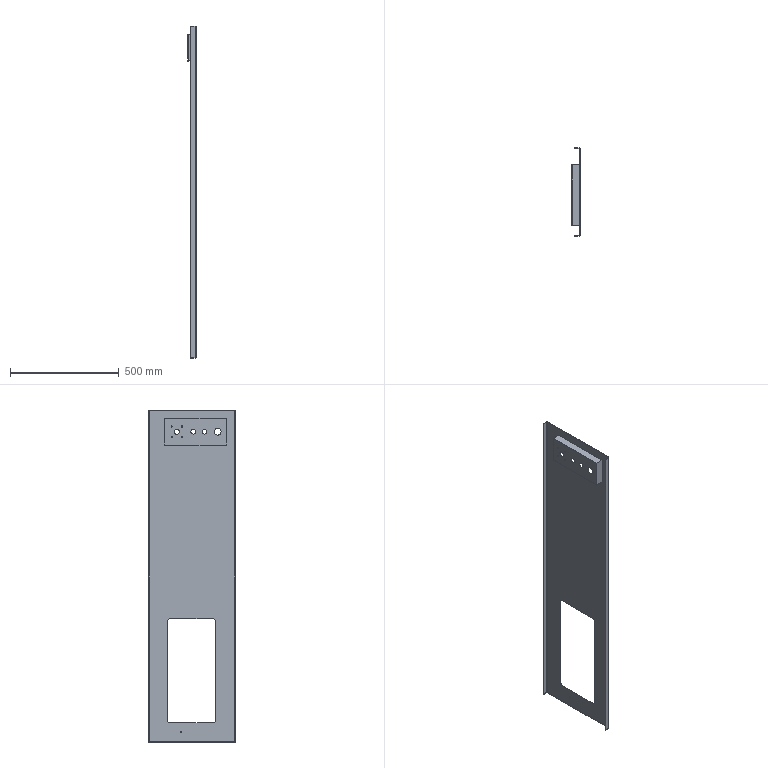Part | STEP file | ASND-0110-E63-HLTP01-003 | 1 solid | 66 faces | box 38 x 405 x 1530 mm | volume 1141633 mm3 | cylinder 32 | plane 28 | other 6 | commonest cylinder face diameters 5.5 x10 6 x6 20 x4 22 x4 7 x2 10 x2